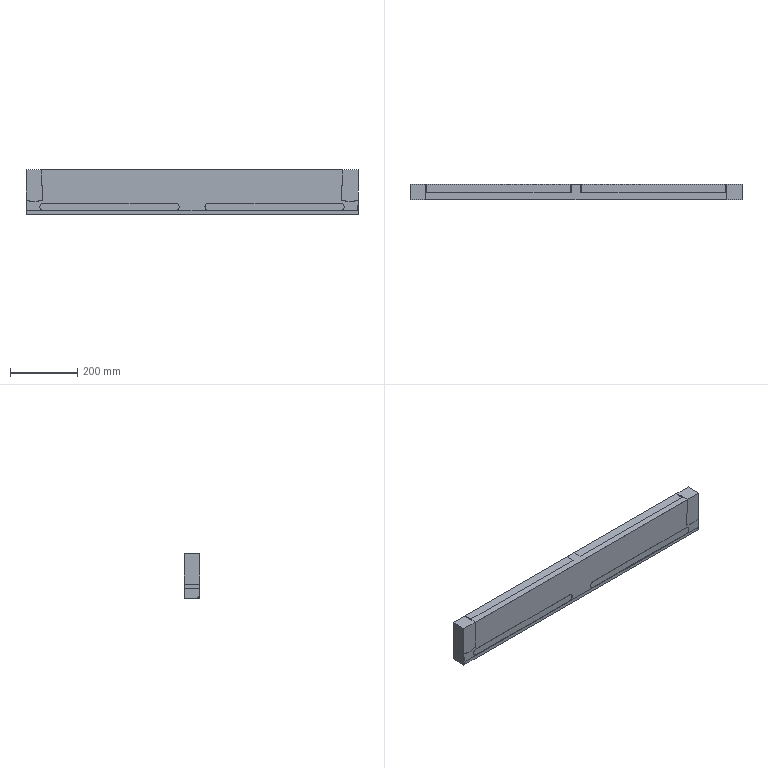NC program | NX | posted with a generic post | part box 987 x 45 x 132.5 mm
Whole program:
N10 G17 G21 G94 G90
(ZLEVEL_PROFILE_COPY_1 , TOOL : D12)
N12 T20 M6
N14 G54
N16 G17 G0 G90 X498.091 Y74.538 B0. C0. S7500 M3
N18 G43 Z30. H20
N20 Z-1.
N22 G94 G1 X496.514 Y73.404 F3000.
N24 G3 X496.021 Y72.311 R1.2
N26 G1 X496.534 Y67.184
N28 X496.619 Y66.359
N30 X499.57 Y36.857
N32 X499.6 Y36.25
N34 Y31.513
N36 X499.597 Y31.459
N38 Y20.192
N40 G3 X500.197 Y19.153 R1.2
N42 G1 X501.779 Y18.239
N44 G0 X501.78 Z-2.
N46 G1 X500.197 Y19.153
N48 G2 X499.597 Y20.192 R1.2
N50 G1 Y31.459
N52 X499.6 Y31.513
N54 Y36.25
N56 X499.57 Y36.857
N58 X496.619 Y66.359
N60 X496.534 Y67.184
N62 X496.021 Y72.311
N64 G2 X496.514 Y73.404 R1.2
N66 G1 X498.091 Y74.538
N68 G0 Z-3.
N70 G1 X496.514 Y73.404
N72 G3 X496.021 Y72.311 R1.2
N74 G1 X496.534 Y67.184
N76 X496.619 Y66.359
N78 X499.57 Y36.857
N80 X499.6 Y36.25
N82 Y31.513
N84 X499.597 Y31.459
N86 Y20.192
N88 G3 X500.197 Y19.153 R1.2
N90 G1 X501.78 Y18.239
N92 G0 Z-4.
N94 G1 X500.197 Y19.153
N96 G2 X499.597 Y20.192 R1.2
N98 G1 X499.6 Y31.513
N100 Y36.25
N102 X499.57 Y36.857
N104 X496.619 Y66.359
N106 X496.534 Y67.184
N108 X496.021 Y72.311
N110 G2 X496.514 Y73.404 R1.2
N112 G1 X498.092 Y74.538
N114 G0 Z-5.
N116 G1 X496.514 Y73.404
N118 G3 X496.021 Y72.311 R1.2
N120 G1 X496.534 Y67.184
N122 X496.619 Y66.359
N124 X499.57 Y36.857
N126 X499.6 Y36.25
N128 X499.597 Y31.459
N130 Y20.192
N132 G3 X500.197 Y19.153 R1.2
N134 G1 X501.78 Y18.239
N136 G0 Z-6.
N138 G1 X500.197 Y19.153
N140 G2 X499.597 Y20.192 R1.2
N142 G1 X499.6 Y31.513
N144 Y36.25
N146 X499.57 Y36.857
N148 X496.619 Y66.359
N150 X496.534 Y67.184
N152 X496.021 Y72.311
N154 G2 X496.515 Y73.404 R1.2
N156 G1 X498.092 Y74.538
N158 G0 Z-7.
N160 G1 X496.515 Y73.404
N162 G3 X496.021 Y72.311 R1.2
N164 G1 X496.534 Y67.184
N166 X496.619 Y66.359
N168 X499.57 Y36.857
N170 X499.6 Y36.25
N172 X499.597 Y31.459
N174 Y20.192
N176 G3 X500.197 Y19.153 R1.2
N178 G1 X501.78 Y18.239
N180 G0 Z-8.
N182 G1 X500.197 Y19.153
N184 G2 X499.597 Y20.192 R1.2
N186 G1 X499.6 Y31.513
N188 Y36.25
N190 X499.57 Y36.857
N192 X496.619 Y66.359
N194 X496.534 Y67.184
N196 X496.021 Y72.311
N198 G2 X496.515 Y73.404 R1.2
N200 G1 X498.092 Y74.538
N202 G0 Z-9.
N204 G1 X496.515 Y73.404
N206 G3 X496.021 Y72.311 R1.2
N208 G1 X496.534 Y67.184
N210 X496.619 Y66.359
N212 X499.57 Y36.857
N214 X499.6 Y36.25
N216 X499.597 Y31.459
N218 Y20.192
N220 G3 X500.197 Y19.153 R1.2
N222 G1 X501.78 Y18.239
N224 G0 Z-10.
N226 G1 X500.197 Y19.153
N228 G2 X499.597 Y20.192 R1.2
N230 G1 X499.6 Y31.513
N232 Y36.25
N234 X499.57 Y36.857
N236 X496.619 Y66.359
N238 X496.534 Y67.184
N240 X496.021 Y72.311
N242 G2 X496.515 Y73.404 R1.2
N244 G1 X498.092 Y74.538
N246 G0 Z-11.
N248 G1 X496.515 Y73.404
N250 G3 X496.021 Y72.311 R1.2
N252 G1 X496.534 Y67.184
N254 X496.619 Y66.359
N256 X499.57 Y36.857
N258 X499.6 Y36.25
N260 X499.597 Y31.459
N262 Y20.192
N264 G3 X500.197 Y19.153 R1.2
N266 G1 X501.78 Y18.239
N268 G0 Z-12.
N270 G1 X500.197 Y19.153
N272 G2 X499.597 Y20.192 R1.2
N274 G1 X499.6 Y31.513
N276 Y36.25
N278 X499.57 Y36.857
N280 X496.619 Y66.359
N282 X496.534 Y67.184
N284 X496.022 Y72.311
N286 G2 X496.515 Y73.405 R1.2
N288 G1 X498.092 Y74.538
N290 G0 Z-13.
N292 G1 X496.515 Y73.405
N294 G3 X496.022 Y72.311 R1.2
N296 G1 X496.535 Y67.184
N298 X496.619 Y66.359
N300 X499.57 Y36.857
N302 X499.6 Y36.25
N304 X499.598 Y31.459
N306 Y20.192
N308 G3 X500.198 Y19.153 R1.2
N310 G1 X501.78 Y18.239
N312 G0 Z-14.
N314 G1 X500.198 Y19.153
N316 G2 X499.598 Y20.192 R1.2
N318 G1 X499.6 Y31.513
N320 Y36.25
N322 X499.57 Y36.857
N324 X496.619 Y66.359
N326 X496.535 Y67.184
N328 X496.022 Y72.311
N330 G2 X496.515 Y73.405 R1.2
N332 G1 X498.092 Y74.538
N334 G0 X498.093 Z-15.
N336 G1 X496.515 Y73.405
N338 G3 X496.022 Y72.311 R1.2
N340 G1 X496.535 Y67.184
N342 X496.619 Y66.359
N344 X499.57 Y36.857
N346 X499.6 Y36.25
N348 X499.598 Y31.459
N350 Y20.192
N352 G3 X500.198 Y19.153 R1.2
N354 G1 X501.78 Y18.239
N356 G0 Z-16.
N358 G1 X500.198 Y19.153
N360 G2 X499.598 Y20.192 R1.2
N362 G1 X499.6 Y31.513
N364 Y36.25
N366 X499.57 Y36.857
N368 X496.619 Y66.359
N370 X496.535 Y67.184
N372 X496.022 Y72.311
N374 G2 X496.515 Y73.405 R1.2
N376 G1 X498.093 Y74.538
N378 G0 X498.092 Y74.539 Z-17.
N380 G1 X496.515 Y73.405
N382 G3 X496.022 Y72.311 R1.2
N384 G1 X496.619 Y66.359
N386 X499.57 Y36.857
N388 X499.6 Y36.25
N390 X499.598 Y31.459
N392 Y20.192
N394 G3 X500.198 Y19.153 R1.2
N396 G1 X501.78 Y18.239
N398 G0 Z-18.
N400 G1 X500.198 Y19.153
N402 G2 X499.598 Y20.192 R1.2
N404 G1 X499.6 Y31.513
N406 Y36.25
N408 X499.57 Y36.857
N410 X496.619 Y66.359
N412 X496.022 Y72.311
N414 G2 X496.515 Y73.405 R1.2
N416 G1 X498.092 Y74.539
N418 G0 X498.097 Y74.542 Z-19.
N420 G1 X496.515 Y73.405
N422 G3 X496.022 Y72.311 R1.2
N424 G1 X496.619 Y66.359
N426 X499.57 Y36.857
N428 X499.6 Y36.25
N430 X499.598 Y31.459
N432 Y20.192
N434 G3 X500.198 Y19.153 R1.2
N436 G1 X501.78 Y18.239
N438 G0 X501.781 Z-20.
N440 G1 X500.198 Y19.153
N442 G2 X499.598 Y20.192 R1.2
N444 G1 X499.6 Y31.513
N446 Y36.25
N448 X499.57 Y36.857
N450 X496.619 Y66.359
N452 X496.022 Y72.311
N454 G2 X496.515 Y73.405 R1.2
N456 G1 X498.097 Y74.542
N458 G0 Y74.541 Z-21.
N460 G1 X496.516 Y73.405
N462 G3 X496.022 Y72.311 R1.2
N464 G1 X496.535 Y67.184
N466 X496.619 Y66.359
N468 X499.57 Y36.857
N470 X499.6 Y36.25
N472 X499.598 Y31.459
N474 Y20.192
N476 G3 X500.198 Y19.153 R1.2
N478 G1 X501.781 Y18.239
N480 G0 Y18.238 Z-22.
N482 G1 X500.198 Y19.153
N484 G2 X499.598 Y20.192 R1.2
N486 G1 X499.6 Y31.513
N488 Y36.25
N490 X499.57 Y36.857
N492 X496.619 Y66.359
N494 X496.535 Y67.184
N496 X496.022 Y72.311
N498 G2 X496.516 Y73.405 R1.2
N500 G1 X498.097 Y74.541
N502 G0 Z-23.
N504 G1 X496.516 Y73.405
N506 G3 X496.023 Y72.311 R1.2
N508 G1 X496.535 Y67.184
N510 X496.619 Y66.359
N512 X499.57 Y36.857
N514 X499.6 Y36.25
N516 Y31.513
N518 X499.598 Y20.192
N520 G3 X500.198 Y19.153 R1.2
N522 G1 X501.781 Y18.238
N524 G0 Z-24.
N526 G1 X500.198 Y19.153
N528 G2 X499.598 Y20.192 R1.2
N530 G1 X499.6 Y31.513
N532 Y36.25
N534 X499.57 Y36.857
N536 X496.619 Y66.359
N538 X496.023 Y72.311
N540 G2 X496.516 Y73.405 R1.2
N542 G1 X498.097 Y74.542
N544 G0 Z-25.
N546 G1 X496.516 Y73.405
N548 G3 X496.023 Y72.311 R1.2
N550 G1 X496.619 Y66.359
N552 X499.57 Y36.857
N554 X499.6 Y36.25
N556 Y31.513
N558 X499.598 Y20.192
N560 G3 X500.198 Y19.153 R1.2
N562 G1 X501.781 Y18.239
N564 G0 Z-26.
N566 G1 X500.198 Y19.153
N568 G2 X499.598 Y20.192 R1.2
N570 G1 X499.6 Y31.513
N572 Y36.25
N574 X499.57 Y36.857
N576 X496.619 Y66.359
N578 X496.023 Y72.311
N580 G2 X496.516 Y73.405 R1.2
N582 G1 X498.097 Y74.542
N584 G0 Z-27.
N586 G1 X496.516 Y73.405
N588 G3 X496.023 Y72.311 R1.2
N590 G1 X496.619 Y66.359
N592 X499.57 Y36.857
N594 X499.6 Y36.25
N596 Y31.513
N598 X499.598 Y20.192
N600 G3 X500.198 Y19.153 R1.2
N602 G1 X501.781 Y18.239
N604 G0 Z-28.
N606 G1 X500.198 Y19.153
N608 G2 X499.599 Y20.192 R1.2
N610 G1 X499.6 Y31.513
N612 Y36.25
N614 X499.57 Y36.857
N616 X496.619 Y66.359
N618 X496.023 Y72.311
N620 G2 X496.516 Y73.405 R1.2
N622 G1 X498.097 Y74.542
N624 G0 Z-29.
N626 G1 X496.516 Y73.405
N628 G3 X496.023 Y72.311 R1.2
N630 G1 X496.619 Y66.359
N632 X499.57 Y36.857
N634 X499.6 Y36.25
N636 Y31.513
N638 X499.599 Y20.192
N640 G3 X500.198 Y19.153 R1.2
N642 G1 X501.781 Y18.239
N644 G0 Z-30.
N646 G1 X500.199 Y19.153
N648 G2 X499.599 Y20.192 R1.2
N650 G1 X499.6 Y31.513
N652 Y36.25
N654 X499.57 Y36.857
N656 X496.619 Y66.359
N658 X496.023 Y72.311
N660 G2 X496.517 Y73.405 R1.2
N662 G1 X498.097 Y74.542
N664 G0 Y74.541 Z-31.
N666 G1 X496.517 Y73.405
N668 G3 X496.023 Y72.311 R1.2
N670 G1 X496.619 Y66.359
N672 X499.57 Y36.857
N674 X499.6 Y36.25
N676 Y31.513
N678 X499.599 Y20.192
N680 G3 X500.199 Y19.153 R1.2
N682 G1 X501.781 Y18.239
N684 G0 Z-32.
N686 G1 X500.199 Y19.153
N688 G2 X499.599 Y20.192 R1.2
N690 G1 X499.6 Y31.513
N692 Y36.25
N694 X499.57 Y36.857
N696 X496.619 Y66.359
N698 X496.023 Y72.311
N700 G2 X496.517 Y73.405 R1.2
N702 G1 X498.097 Y74.541
N704 G0 Z-33.
N706 G1 X496.517 Y73.405
N708 G3 X496.023 Y72.311 R1.2
N710 G1 X496.619 Y66.359
N712 X499.57 Y36.857
N714 X499.6 Y36.25
N716 Y31.513
N718 X499.599 Y20.192
N720 G3 X500.199 Y19.153 R1.2
N722 G1 X501.781 Y18.239
N724 G0 Z-34.
N726 G1 X500.199 Y19.153
N728 G2 X499.599 Y20.192 R1.2
N730 G1 X499.6 Y31.513
N732 Y36.25
N734 X499.57 Y36.857
N736 X496.619 Y66.359
N738 X496.024 Y72.311
N740 G2 X496.517 Y73.405 R1.2
N742 G1 X498.097 Y74.541
N744 G0 Z-35.
N746 G1 X496.517 Y73.405
N748 G3 X496.024 Y72.311 R1.2
N750 G1 X496.619 Y66.359
N752 X499.57 Y36.857
N754 X499.6 Y36.25
N756 Y31.513
N758 X499.599 Y20.192
N760 G3 X500.199 Y19.153 R1.2
N762 G1 X501.781 Y18.239
N764 G0 Z-36.
N766 G1 X500.199 Y19.153
N768 G2 X499.599 Y20.192 R1.2
N770 G1 X499.6 Y31.513
N772 Y36.25
N774 X499.57 Y36.857
N776 X496.619 Y66.359
N778 X496.024 Y72.311
N780 G2 X496.517 Y73.405 R1.2
N782 G1 X498.098 Y74.541
N784 G0 X498.094 Y74.539 Z-37.
N786 G1 X496.517 Y73.405
N788 G3 X496.024 Y72.311 R1.2
N790 G1 X496.619 Y66.359
N792 X499.57 Y36.857
N794 X499.6 Y36.25
N796 Y31.513
N798 X499.599 Y20.192
N800 G3 X500.199 Y19.153 R1.2
N802 G1 X501.781 Y18.239
N804 G0 Z-38.
N806 G1 X500.199 Y19.153
N808 G2 X499.599 Y20.192 R1.2
N810 G1 X499.6 Y31.513
N812 Y36.25
N814 X499.57 Y36.857
N816 X496.619 Y66.359
N818 X496.024 Y72.311
N820 G2 X496.517 Y73.405 R1.2
N822 G1 X498.094 Y74.539
N824 G0 Y74.538 Z-39.
N826 G1 X496.518 Y73.405
N828 G3 X496.024 Y72.311 R1.2
N830 G1 X496.619 Y66.359
N832 X499.57 Y36.857
N834 X499.6 Y36.25
N836 Y31.513
N838 X499.599 Y20.192
N840 G3 X500.199 Y19.152 R1.2
N842 G1 X501.781 Y18.239
N844 G0 Z-40.
N846 G1 X500.199 Y19.152
N848 G2 X499.599 Y20.192 R1.2
N850 G1 X499.6 Y31.513
N852 Y36.25
N854 X499.57 Y36.857
N856 X496.619 Y66.359
N858 X496.024 Y72.311
N860 G2 X496.518 Y73.405 R1.2
N862 G1 X498.095 Y74.538
N864 G0 Z-41.
N866 G1 X496.518 Y73.405
N868 G3 X496.024 Y72.311 R1.2
N870 G1 X496.619 Y66.359
N872 X499.57 Y36.857
N874 X499.6 Y36.25
N876 Y31.513
N878 X499.599 Y20.192
N880 G3 X500.199 Y19.152 R1.2
N882 G1 X501.781 Y18.239
N884 G0 X501.782 Z-42.
N886 G1 X500.199 Y19.152
N888 G2 X499.599 Y20.192 R1.2
N890 G1 X499.6 Y31.513
N892 Y36.25
N894 X499.57 Y36.857
N896 X496.619 Y66.359
N898 X496.024 Y72.311
N900 G2 X496.518 Y73.405 R1.2
N902 G1 X498.095 Y74.538
N904 G0 Z-43.
N906 G1 X496.518 Y73.405
N908 G3 X496.024 Y72.311 R1.2
N910 G1 X496.619 Y66.359
N912 X499.57 Y36.857
N914 X499.6 Y36.25
N916 Y31.513
N918 X499.599 Y20.192
N920 G3 X500.199 Y19.152 R1.2
N922 G1 X501.782 Y18.239
N924 G0 Z-44.
N926 G1 X500.199 Y19.152
N928 G2 X499.6 Y20.192 R1.2
N930 G1 Y31.513
N932 Y36.25
N934 X499.57 Y36.857
N936 X496.619 Y66.359
N938 X496.024 Y72.311
N940 G2 X496.518 Y73.405 R1.2
N942 G1 X498.095 Y74.538
N944 G0 Z-45.
N946 G1 X496.518 Y73.405
N948 G3 X496.024 Y72.311 R1.2
N950 G1 X496.619 Y66.359
N952 X499.57 Y36.857
N954 X499.6 Y36.25
N956 Y31.513
N958 Y20.192
N960 G3 X500.2 Y19.152 R1.2
N962 G1 X501.782 Y18.239
N964 G0 Z30.
N966 X-501.779
N968 Z-1.
N970 G1 X-500.197 Y19.153
N972 G3 X-499.597 Y20.192 R1.2
N974 G1 Y25.852
N976 X-499.542 Y25.913
N978 G2 X-499.54 Y27.606 R6.1
N980 G1 X-499.597 Y27.668
N982 Y31.459
N984 X-499.6 Y31.513
N986 Y36.25
N988 X-499.57 Y36.857
N990 X-496.619 Y66.359
N992 X-496.477 Y67.194
N994 X-496.528 Y67.237
N996 X-496.021 Y72.311
N998 G3 X-496.514 Y73.404 R1.2
N1000 G1 X-498.098 Y74.543
N1002 G0 Z-2.
N1004 G1 X-496.514 Y73.404
N1006 G2 X-496.021 Y72.311 R1.2
N1008 G1 X-496.528 Y67.237
N1010 X-496.477 Y67.194
N1012 X-496.619 Y66.359
N1014 X-499.57 Y36.857
N1016 X-499.6 Y36.25
N1018 Y31.513
N1020 X-499.597 Y31.459
N1022 Y27.668
N1024 X-499.54 Y27.606
N1026 G3 X-499.542 Y25.913 R6.1
N1028 G1 X-499.597 Y25.852
N1030 Y20.192
N1032 G2 X-500.197 Y19.153 R1.2
N1034 G1 X-501.78 Y18.239
N1036 G0 Z-3.
N1038 G1 X-500.197 Y19.153
N1040 G3 X-499.597 Y20.192 R1.2
N1042 G1 Y25.852
N1044 X-499.542 Y25.913
N1046 G2 X-499.54 Y27.606 R6.1
N1048 G1 X-499.597 Y27.668
N1050 Y31.459
N1052 X-499.6 Y31.513
N1054 Y36.25
N1056 X-499.57 Y36.857
N1058 X-496.619 Y66.359
N1060 X-496.477 Y67.194
N1062 X-496.529 Y67.237
N1064 X-496.021 Y72.311
N1066 G3 X-496.514 Y73.404 R1.2
N1068 G1 X-498.098 Y74.543
N1070 G0 Z-4.
N1072 G1 X-496.514 Y73.404
N1074 G2 X-496.021 Y72.311 R1.2
N1076 G1 X-496.529 Y67.237
N1078 X-496.477 Y67.194
N1080 X-496.619 Y66.359
N1082 X-499.57 Y36.857
N1084 X-499.6 Y36.25
N1086 X-499.597 Y31.459
N1088 Y27.668
N1090 X-499.54 Y27.606
N1092 G3 X-499.542 Y25.913 R6.1
N1094 G1 X-499.597 Y25.852
N1096 Y20.192
N1098 G2 X-500.197 Y19.153 R1.2
N1100 G1 X-501.78 Y18.239
N1102 G0 Z-5.
N1104 G1 X-500.197 Y19.153
N1106 G3 X-499.597 Y20.192 R1.2
N1108 G1 Y25.852
N1110 X-499.542 Y25.913
N1112 G2 X-499.54 Y27.606 R6.1
N1114 G1 X-499.597 Y27.668
N1116 X-499.6 Y31.513
N1118 Y36.25
N1120 X-499.57 Y36.857
N1122 X-496.619 Y66.359
N1124 X-496.477 Y67.194
N1126 X-496.529 Y67.237
N1128 X-496.021 Y72.311
N1130 G3 X-496.514 Y73.404 R1.2
N1132 G1 X-498.098 Y74.543
N1134 G0 Z-6.
N1136 G1 X-496.515 Y73.404
N1138 G2 X-496.021 Y72.311 R1.2
N1140 G1 X-496.529 Y67.237
N1142 X-496.477 Y67.194
N1144 X-496.619 Y66.359
N1146 X-499.57 Y36.857
N1148 X-499.6 Y36.25
N1150 X-499.597 Y31.459
N1152 Y27.668
N1154 X-499.54 Y27.606
N1156 G3 X-499.542 Y25.913 R6.1
N1158 G1 X-499.597 Y25.852
N1160 Y20.192
N1162 G2 X-500.197 Y19.153 R1.2
N1164 G1 X-501.78 Y18.239
N1166 G0 Z-7.
N1168 G1 X-500.197 Y19.153
N1170 G3 X-499.597 Y20.192 R1.2
N1172 G1 Y25.852
N1174 X-499.542 Y25.913
N1176 G2 X-499.54 Y27.606 R6.1
N1178 G1 X-499.597 Y27.668
N1180 X-499.6 Y31.513
N1182 Y36.25
N1184 X-499.57 Y36.857
N1186 X-496.619 Y66.359
N1188 X-496.477 Y67.194
N1190 X-496.529 Y67.237
N1192 X-496.021 Y72.311
N1194 G3 X-496.515 Y73.404 R1.2
N1196 G1 X-498.098 Y74.543
N1198 G0 Z-8.
N1200 G1 X-496.515 Y73.404
N1202 G2 X-496.021 Y72.311 R1.2
N1204 G1 X-496.529 Y67.237
N1206 X-496.477 Y67.194
N1208 X-496.619 Y66.359
N1210 X-499.57 Y36.857
N1212 X-499.6 Y36.25
N1214 X-499.597 Y31.459
N1216 Y27.668
N1218 X-499.54 Y27.606
N1220 G3 X-499.542 Y25.913 R6.1
N1222 G1 X-499.597 Y25.852
N1224 Y20.192
N1226 G2 X-500.197 Y19.153 R1.2
N1228 G1 X-501.78 Y18.239
N1230 G0 Z-9.
N1232 G1 X-500.197 Y19.153
N1234 G3 X-499.597 Y20.192 R1.2
N1236 G1 Y25.852
N1238 X-499.542 Y25.913
N1240 G2 X-499.54 Y27.606 R6.1
N1242 G1 X-499.597 Y27.668
N1244 X-499.6 Y31.513
N1246 Y36.25
N1248 X-499.57 Y36.857
N1250 X-496.619 Y66.359
N1252 X-496.477 Y67.194
N1254 X-496.529 Y67.237
N1256 X-496.021 Y72.311
N1258 G3 X-496.515 Y73.404 R1.2
N1260 G1 X-498.099 Y74.543
N1262 G0 Z-10.
N1264 G1 X-496.515 Y73.404
N1266 G2 X-496.021 Y72.311 R1.2
N1268 G1 X-496.529 Y67.237
N1270 X-496.477 Y67.194
N1272 X-496.619 Y66.359
N1274 X-499.57 Y36.857
N1276 X-499.6 Y36.25
N1278 X-499.597 Y31.459
N1280 Y27.668
N1282 X-499.54 Y27.606
N1284 G3 X-499.542 Y25.913 R6.1
N1286 G1 X-499.597 Y25.852
N1288 Y20.192
N1290 G2 X-500.197 Y19.153 R1.2
N1292 G1 X-501.78 Y18.239
N1294 G0 Z-11.
N1296 G1 X-500.197 Y19.153
N1298 G3 X-499.597 Y20.192 R1.2
N1300 G1 Y25.852
N1302 X-499.542 Y25.913
N1304 G2 X-499.54 Y27.606 R6.1
N1306 G1 X-499.597 Y27.668
N1308 X-499.6 Y31.513
N1310 Y36.25
N1312 X-499.57 Y36.857
N1314 X-496.619 Y66.359
N1316 X-496.477 Y67.194
N1318 X-496.529 Y67.237
N1320 X-496.021 Y72.311
N1322 G3 X-496.515 Y73.404 R1.2
N1324 G1 X-498.099 Y74.543
N1326 G0 Z-12.
N1328 G1 X-496.515 Y73.405
N1330 G2 X-496.022 Y72.311 R1.2
N1332 G1 X-496.529 Y67.237
N1334 X-496.477 Y67.194
N1336 X-496.619 Y66.359
N1338 X-499.57 Y36.857
N1340 X-499.6 Y36.25
N1342 X-499.598 Y31.459
N1344 Y27.668
N1346 X-499.54 Y27.606
N1348 G3 X-499.542 Y25.913 R6.1
N1350 G1 X-499.598 Y25.852
N1352 X-499.597 Y20.192
N1354 G2 X-500.197 Y19.153 R1.2
N1356 G1 X-501.78 Y18.239
N1358 G0 Z-13.
N1360 G1 X-500.198 Y19.153
N1362 G3 X-499.598 Y20.192 R1.2
N1364 G1 Y25.852
N1366 X-499.542 Y25.913
N1368 G2 X-499.54 Y27.606 R6.1
N1370 G1 X-499.598 Y27.668
N1372 X-499.6 Y31.513
N1374 Y36.25
N1376 X-499.57 Y36.857
N1378 X-496.619 Y66.359
N1380 X-496.477 Y67.194
N1382 X-496.529 Y67.237
N1384 X-496.022 Y72.311
N1386 G3 X-496.515 Y73.405 R1.2
N1388 G1 X-498.099 Y74.543
N1390 G0 Z-14.
N1392 G1 X-496.515 Y73.405
N1394 G2 X-496.022 Y72.311 R1.2
N1396 G1 X-496.529 Y67.237
N1398 X-496.477 Y67.194
N1400 X-496.619 Y66.359
N1402 X-499.57 Y36.857
N1404 X-499.6 Y36.25
N1406 X-499.598 Y31.459
N1408 Y27.668
N1410 X-499.54 Y27.606
N1412 G3 X-499.542 Y25.913 R6.1
N1414 G1 X-499.598 Y25.852
N1416 Y20.192
N1418 G2 X-500.198 Y19.153 R1.2
N1420 G1 X-501.78 Y18.239
N1422 G0 Z-15.
N1424 G1 X-500.198 Y19.153
N1426 G3 X-499.598 Y20.192 R1.2
N1428 G1 Y25.852
N1430 X-499.542 Y25.913
N1432 G2 X-499.54 Y27.606 R6.1
N1434 G1 X-499.598 Y27.668
N1436 X-499.6 Y31.513
N1438 Y36.25
N1440 X-499.57 Y36.857
N1442 X-496.619 Y66.359
N1444 X-496.477 Y67.194
N1446 X-496.529 Y67.237
N1448 X-496.022 Y72.311
N1450 G3 X-496.515 Y73.405 R1.2
N1452 G1 X-498.099 Y74.543
N1454 G0 Z-16.
N1456 G1 X-496.515 Y73.405
N1458 G2 X-496.022 Y72.311 R1.2
N1460 G1 X-496.529 Y67.237
N1462 X-496.477 Y67.194
N1464 X-496.619 Y66.359
N1466 X-499.57 Y36.857
N1468 X-499.6 Y36.25
N1470 X-499.598 Y31.459
N1472 Y27.668
N1474 X-499.54 Y27.606
N1476 G3 X-499.542 Y25.913 R6.1
N1478 G1 X-499.598 Y25.852
N1480 Y20.192
N1482 G2 X-500.198 Y19.153 R1.2
N1484 G1 X-501.78 Y18.239
N1486 G0 Z-17.
N1488 G1 X-500.198 Y19.153
N1490 G3 X-499.598 Y20.192 R1.2
N1492 G1 Y25.852
N1494 X-499.542 Y25.913
N1496 G2 X-499.54 Y27.606 R6.1
N1498 G1 X-499.598 Y27.668
N1500 X-499.6 Y31.513
N1502 Y36.25
N1504 X-499.57 Y36.857
N1506 X-496.619 Y66.359
N1508 X-496.477 Y67.194
N1510 X-496.53 Y67.237
N1512 X-496.022 Y72.311
N1514 G3 X-496.516 Y73.405 R1.2
N1516 G1 X-498.099 Y74.543
N1518 G0 Z-18.
N1520 G1 X-496.516 Y73.405
N1522 G2 X-496.022 Y72.311 R1.2
N1524 G1 X-496.53 Y67.237
N1526 X-496.477 Y67.194
N1528 X-496.619 Y66.359
N1530 X-499.57 Y36.857
N1532 X-499.6 Y36.25
N1534 X-499.598 Y31.459
N1536 Y27.668
N1538 X-499.54 Y27.606
N1540 G3 X-499.542 Y25.913 R6.1
N1542 G1 X-499.598 Y25.852
N1544 Y20.192
N1546 G2 X-500.198 Y19.153 R1.2
N1548 G1 X-501.78 Y18.239
N1550 G0 Z-19.
N1552 G1 X-500.198 Y19.153
N1554 G3 X-499.598 Y20.192 R1.2
N1556 G1 Y25.852
N1558 X-499.542 Y25.913
N1560 G2 X-499.54 Y27.606 R6.1
N1562 G1 X-499.598 Y27.668
N1564 X-499.6 Y31.513
N1566 Y36.25
N1568 X-499.57 Y36.857
N1570 X-496.619 Y66.359
N1572 X-496.477 Y67.194
N1574 X-496.53 Y67.237
N1576 X-496.022 Y72.311
N1578 G3 X-496.516 Y73.405 R1.2
N1580 G1 X-498.099 Y74.543
N1582 G0 Z-20.
N1584 G1 X-496.516 Y73.405
N1586 G2 X-496.022 Y72.311 R1.2
N1588 G1 X-496.53 Y67.237
N1590 X-496.477 Y67.194
N1592 X-496.619 Y66.359
N1594 X-499.57 Y36.857
N1596 X-499.6 Y36.25
N1598 X-499.598 Y31.459
N1600 Y27.668
N1602 X-499.54 Y27.606
N1604 G3 X-499.542 Y25.913 R6.1
N1606 G1 X-499.598 Y25.852
N1608 Y20.192
N1610 G2 X-500.198 Y19.153 R1.2
N1612 G1 X-501.781 Y18.239
N1614 G0 Z-21.
N1616 G1 X-500.198 Y19.153
N1618 G3 X-499.598 Y20.192 R1.2
N1620 G1 Y25.852
N1622 X-499.542 Y25.913
N1624 G2 X-499.54 Y27.606 R6.1
N1626 G1 X-499.598 Y27.668
N1628 X-499.6 Y31.513
N1630 Y36.25
N1632 X-499.57 Y36.857
N1634 X-496.619 Y66.359
N1636 X-496.477 Y67.194
N1638 X-496.53 Y67.237
N1640 X-496.022 Y72.311
N1642 G3 X-496.516 Y73.405 R1.2
N1644 G1 X-498.099 Y74.543
N1646 G0 X-498.1 Z-22.
N1648 G1 X-496.516 Y73.405
N1650 G2 X-496.022 Y72.311 R1.2
N1652 G1 X-496.53 Y67.237
N1654 X-496.477 Y67.194
N1656 X-496.619 Y66.359
N1658 X-499.57 Y36.857
N1660 X-499.6 Y36.25
N1662 Y31.513
N1664 X-499.598 Y27.668
N1666 X-499.54 Y27.606
N1668 G3 X-499.542 Y25.913 R6.1
N1670 G1 X-499.598 Y25.852
N1672 Y20.192
N1674 G2 X-500.198 Y19.153 R1.2
N1676 G1 X-501.781 Y18.239
N1678 G0 Z-23.
N1680 G1 X-500.198 Y19.153
N1682 G3 X-499.598 Y20.192 R1.2
N1684 G1 Y25.852
N1686 X-499.542 Y25.913
N1688 G2 X-499.54 Y27.606 R6.1
N1690 G1 X-499.598 Y27.668
N1692 X-499.6 Y31.513
N1694 Y36.25
N1696 X-499.57 Y36.857
N1698 X-496.619 Y66.359
N1700 X-496.477 Y67.194
N1702 X-496.53 Y67.237
N1704 X-496.023 Y72.311
N1706 G3 X-496.516 Y73.405 R1.2
N1708 G1 X-498.1 Y74.543
N1710 G0 Z-24.
N1712 G1 X-496.516 Y73.405
N1714 G2 X-496.023 Y72.311 R1.2
N1716 G1 X-496.53 Y67.237
N1718 X-496.477 Y67.194
N1720 X-496.619 Y66.359
N1722 X-499.57 Y36.857
N1724 X-499.6 Y36.25
N1726 Y31.513
N1728 X-499.598 Y27.668
N1730 X-499.54 Y27.606
N1732 G3 X-499.542 Y25.913 R6.1
N1734 G1 X-499.598 Y25.852
N1736 Y20.192
N1738 G2 X-500.198 Y19.153 R1.2
N1740 G1 X-501.781 Y18.239
N1742 G0 Z-25.
N1744 G1 X-500.198 Y19.153
N1746 G3 X-499.598 Y20.192 R1.2
N1748 G1 Y25.852
N1750 X-499.542 Y25.913
N1752 G2 X-499.54 Y27.606 R6.1
N1754 G1 X-499.598 Y27.668
N1756 X-499.6 Y31.513
N1758 Y36.25
N1760 X-499.57 Y36.857
N1762 X-496.619 Y66.359
N1764 X-496.477 Y67.194
N1766 X-496.53 Y67.237
N1768 X-496.023 Y72.311
N1770 G3 X-496.516 Y73.405 R1.2
N1772 G1 X-498.1 Y74.543
N1774 G0 Z-26.
N1776 G1 X-496.516 Y73.405
N1778 G2 X-496.023 Y72.311 R1.2
N1780 G1 X-496.53 Y67.237
N1782 X-496.477 Y67.194
N1784 X-496.619 Y66.359
N1786 X-499.57 Y36.857
N1788 X-499.6 Y36.25
N1790 Y31.513
N1792 X-499.598 Y27.668
N1794 X-499.54 Y27.606
N1796 G3 X-499.542 Y25.913 R6.1
N1798 G1 X-499.598 Y25.852
N1800 Y20.192
N1802 G2 X-500.198 Y19.153 R1.2
N1804 G1 X-501.781 Y18.239
N1806 G0 Z-27.
N1808 G1 X-500.198 Y19.153
N1810 G3 X-499.598 Y20.192 R1.2
N1812 G1 Y25.852
N1814 X-499.542 Y25.913
N1816 G2 X-499.54 Y27.606 R6.1
N1818 G1 X-499.598 Y27.668
N1820 X-499.6 Y31.513
N1822 Y36.25
N1824 X-499.57 Y36.857
N1826 X-496.619 Y66.359
N1828 X-496.477 Y67.194
N1830 X-496.53 Y67.237
N1832 X-496.023 Y72.311
N1834 G3 X-496.517 Y73.405 R1.2
N1836 G1 X-498.1 Y74.543
N1838 G0 Z-28.
N1840 G1 X-496.517 Y73.405
N1842 G2 X-496.023 Y72.311 R1.2
N1844 G1 X-496.53 Y67.237
N1846 X-496.477 Y67.194
N1848 X-496.619 Y66.359
N1850 X-499.57 Y36.857
N1852 X-499.6 Y36.25
N1854 Y31.513
N1856 X-499.599 Y27.668
N1858 X-499.54 Y27.606
N1860 G3 X-499.542 Y25.913 R6.1
N1862 G1 X-499.599 Y25.852
N1864 Y20.192
N1866 G2 X-500.199 Y19.153 R1.2
N1868 G1 X-501.781 Y18.239
N1870 G0 Z-29.
N1872 G1 X-500.199 Y19.153
N1874 G3 X-499.599 Y20.192 R1.2
N1876 G1 Y25.852
N1878 X-499.542 Y25.913
N1880 G2 X-499.54 Y27.606 R6.1
N1882 G1 X-499.599 Y27.668
N1884 X-499.6 Y31.513
N1886 Y36.25
N1888 X-499.57 Y36.857
N1890 X-496.619 Y66.359
N1892 X-496.477 Y67.194
N1894 X-496.53 Y67.237
N1896 X-496.023 Y72.311
N1898 G3 X-496.517 Y73.405 R1.2
N1900 G1 X-498.1 Y74.543
N1902 G0 Z-30.
N1904 G1 X-496.517 Y73.405
N1906 G2 X-496.023 Y72.311 R1.2
N1908 G1 X-496.53 Y67.237
N1910 X-496.477 Y67.194
N1912 X-496.619 Y66.359
N1914 X-499.57 Y36.857
N1916 X-499.6 Y36.25
N1918 Y31.513
N1920 X-499.599 Y27.668
N1922 X-499.54 Y27.606
N1924 G3 X-499.542 Y25.913 R6.1
N1926 G1 X-499.599 Y25.852
N1928 Y20.192
N1930 G2 X-500.199 Y19.153 R1.2
N1932 G1 X-501.781 Y18.239
N1934 G0 Z-31.
N1936 G1 X-500.199 Y19.153
N1938 G3 X-499.599 Y20.192 R1.2
N1940 G1 Y25.852
N1942 X-499.542 Y25.913
N1944 G2 X-499.54 Y27.606 R6.1
N1946 G1 X-499.599 Y27.668
N1948 X-499.6 Y31.513
N1950 Y36.25
N1952 X-499.57 Y36.857
N1954 X-496.619 Y66.359
N1956 X-496.477 Y67.194
N1958 X-496.53 Y67.237
N1960 X-496.023 Y72.311
N1962 G3 X-496.517 Y73.405 R1.2
N1964 G1 X-498.1 Y74.543
N1966 G0 Z-32.
N1968 G1 X-496.517 Y73.405
N1970 G2 X-496.023 Y72.311 R1.2
N1972 G1 X-496.531 Y67.237
N1974 X-496.477 Y67.194
N1976 X-496.619 Y66.359
N1978 X-499.57 Y36.857
N1980 X-499.6 Y36.25
N1982 Y31.513
N1984 X-499.599 Y27.668
N1986 X-499.54 Y27.606
N1988 G3 X-499.542 Y25.913 R6.1
N1990 G1 X-499.599 Y25.852
N1992 Y20.192
N1994 G2 X-500.199 Y19.153 R1.2
N1996 G1 X-501.781 Y18.239
N1998 G0 Z-33.
N2000 G1 X-500.199 Y19.153
N2002 G3 X-499.599 Y20.192 R1.2
N2004 G1 Y25.852
N2006 X-499.542 Y25.913
N2008 G2 X-499.54 Y27.606 R6.1
N2010 G1 X-499.599 Y27.668
N2012 X-499.6 Y31.513
N2014 Y36.25
N2016 X-499.57 Y36.857
N2018 X-496.619 Y66.359
N2020 X-496.477 Y67.194
N2022 X-496.531 Y67.237
N2024 X-496.023 Y72.311
N2026 G3 X-496.517 Y73.405 R1.2
N2028 G1 X-498.1 Y74.543
N2030 G0 Z-34.
N2032 G1 X-496.517 Y73.405
N2034 G2 X-496.024 Y72.311 R1.2
N2036 G1 X-496.531 Y67.237
N2038 X-496.477 Y67.194
N2040 X-496.619 Y66.359
N2042 X-499.57 Y36.857
N2044 X-499.6 Y36.25
N2046 Y31.513
N2048 X-499.599 Y27.668
N2050 X-499.54 Y27.606
N2052 G3 X-499.542 Y25.913 R6.1
N2054 G1 X-499.599 Y25.852
N2056 Y20.192
N2058 G2 X-500.199 Y19.153 R1.2
N2060 G1 X-501.781 Y18.239
N2062 G0 Z-35.
N2064 G1 X-500.199 Y19.153
N2066 G3 X-499.599 Y20.192 R1.2
N2068 G1 Y25.852
N2070 X-499.542 Y25.913
N2072 G2 X-499.54 Y27.606 R6.1
N2074 G1 X-499.599 Y27.668
N2076 X-499.6 Y31.513
N2078 Y36.25
N2080 X-499.57 Y36.857
N2082 X-496.619 Y66.359
N2084 X-496.477 Y67.194
N2086 X-496.531 Y67.237
N2088 X-496.024 Y72.311
N2090 G3 X-496.517 Y73.405 R1.2
N2092 G1 X-498.101 Y74.543
N2094 G0 Z-36.
N2096 G1 X-496.517 Y73.405
N2098 G2 X-496.024 Y72.311 R1.2
N2100 G1 X-496.531 Y67.237
N2102 X-496.477 Y67.194
N2104 X-496.619 Y66.359
N2106 X-499.57 Y36.857
N2108 X-499.6 Y36.25
N2110 Y31.513
N2112 X-499.599 Y27.668
N2114 X-499.54 Y27.606
N2116 G3 X-499.542 Y25.913 R6.1
N2118 G1 X-499.599 Y25.852
N2120 Y20.192
N2122 G2 X-500.199 Y19.153 R1.2
N2124 G1 X-501.781 Y18.239
N2126 G0 Z-37.
N2128 G1 X-500.199 Y19.153
N2130 G3 X-499.599 Y20.192 R1.2
N2132 G1 Y25.852
N2134 X-499.542 Y25.913
N2136 G2 X-499.54 Y27.606 R6.1
N2138 G1 X-499.599 Y27.668
N2140 X-499.6 Y31.513
N2142 Y36.25
N2144 X-499.57 Y36.857
N2146 X-496.619 Y66.359
N2148 X-496.477 Y67.194
N2150 X-496.531 Y67.237
N2152 X-496.024 Y72.311
N2154 G3 X-496.517 Y73.405 R1.2
N2156 G1 X-498.101 Y74.543
N2158 G0 Z-38.
N2160 G1 X-496.518 Y73.405
N2162 G2 X-496.024 Y72.311 R1.2
N2164 G1 X-496.531 Y67.237
N2166 X-496.477 Y67.194
N2168 X-496.619 Y66.359
N2170 X-499.57 Y36.857
N2172 X-499.6 Y36.25
N2174 Y31.513
N2176 X-499.599 Y27.668
N2178 X-499.54 Y27.606
N2180 G3 X-499.542 Y25.913 R6.1
N2182 G1 X-499.599 Y25.852
N2184 Y20.192
N2186 G2 X-500.199 Y19.153 R1.2
N2188 G1 X-501.781 Y18.239
N2190 G0 Z-39.
N2192 G1 X-500.199 Y19.153
N2194 G3 X-499.599 Y20.192 R1.2
N2196 G1 Y25.852
N2198 X-499.542 Y25.913
N2200 G2 X-499.54 Y27.606 R6.1
N2202 G1 X-499.599 Y27.668
N2204 X-499.6 Y31.513
N2206 Y36.25
N2208 X-499.57 Y36.857
N2210 X-496.619 Y66.359
N2212 X-496.477 Y67.194
N2214 X-496.531 Y67.237
N2216 X-496.024 Y72.311
N2218 G3 X-496.518 Y73.405 R1.2
N2220 G1 X-498.101 Y74.543
N2222 G0 Z-40.
N2224 G1 X-496.518 Y73.405
N2226 G2 X-496.024 Y72.311 R1.2
N2228 G1 X-496.531 Y67.237
N2230 X-496.477 Y67.194
N2232 X-496.619 Y66.359
N2234 X-499.57 Y36.857
N2236 X-499.6 Y36.25
N2238 Y31.513
N2240 X-499.599 Y27.668
N2242 X-499.54 Y27.606
N2244 G3 X-499.542 Y25.913 R6.1
N2246 G1 X-499.599 Y25.852
N2248 Y20.192
N2250 G2 X-500.199 Y19.153 R1.2
N2252 G1 X-501.781 Y18.239
N2254 G0 Z-41.
N2256 G1 X-500.199 Y19.153
N2258 G3 X-499.599 Y20.192 R1.2
N2260 G1 Y25.852
N2262 X-499.542 Y25.913
N2264 G2 X-499.54 Y27.606 R6.1
N2266 G1 X-499.599 Y27.668
N2268 X-499.6 Y31.513
N2270 Y36.25
N2272 X-499.57 Y36.857
N2274 X-496.619 Y66.359
N2276 X-496.477 Y67.194
N2278 X-496.531 Y67.237
N2280 X-496.024 Y72.311
N2282 G3 X-496.518 Y73.405 R1.2
N2284 G1 X-498.101 Y74.543
N2286 G0 Z-42.
N2288 G1 X-496.518 Y73.405
N2290 G2 X-496.024 Y72.311 R1.2
N2292 G1 X-496.531 Y67.237
N2294 X-496.477 Y67.194
N2296 X-496.619 Y66.359
N2298 X-499.57 Y36.857
N2300 X-499.6 Y36.25
N2302 Y31.513
N2304 X-499.599 Y27.668
N2306 X-499.54 Y27.606
N2308 G3 X-499.542 Y25.913 R6.1
N2310 G1 X-499.599 Y25.852
N2312 Y20.192
N2314 G2 X-500.199 Y19.153 R1.2
N2316 G1 X-501.782 Y18.239
N2318 G0 Z-43.
N2320 G1 X-500.199 Y19.153
N2322 G3 X-499.599 Y20.192 R1.2
N2324 G1 Y25.852
N2326 X-499.542 Y25.913
N2328 G2 X-499.54 Y27.606 R6.1
N2330 G1 X-499.599 Y27.668
N2332 X-499.6 Y31.513
N2334 Y36.25
N2336 X-499.57 Y36.857
N2338 X-496.619 Y66.359
N2340 X-496.477 Y67.194
N2342 X-496.531 Y67.237
N2344 X-496.024 Y72.311
N2346 G3 X-496.518 Y73.405 R1.2
N2348 G1 X-498.101 Y74.543
N2350 G0 Z-44.
N2352 G1 X-496.518 Y73.405
N2354 G2 X-496.024 Y72.311 R1.2
N2356 G1 X-496.531 Y67.237
N2358 X-496.477 Y67.194
N2360 X-496.619 Y66.359
N2362 X-499.57 Y36.857
N2364 X-499.6 Y36.25
N2366 Y31.513
N2368 Y27.668
N2370 X-499.54 Y27.606
N2372 G3 X-499.542 Y25.913 R6.1
N2374 G1 X-499.6 Y25.852
N2376 Y20.192
N2378 G2 X-500.2 Y19.153 R1.2
N2380 G1 X-501.782 Y18.239
N2382 G0 Z-45.
N2384 G1 X-500.2 Y19.153
N2386 G3 X-499.6 Y20.192 R1.2
N2388 G1 Y25.852
N2390 X-499.542 Y25.913
N2392 G2 X-499.54 Y27.606 R6.1
N2394 G1 X-499.6 Y27.668
N2396 Y31.513
N2398 Y36.25
N2400 X-499.57 Y36.857
N2402 X-496.619 Y66.359
N2404 X-496.477 Y67.194
N2406 X-496.531 Y67.237
N2408 X-496.024 Y72.311
N2410 G3 X-496.518 Y73.405 R1.2
N2412 G1 X-498.101 Y74.543
N2414 G0 Z30.
N2416 M5
(111 , TOOL : D12JING)
N2418 T21 M6
N2420 G54
N2422 G17 G0 G90 X489.819 Y77.751 B0. C0. S6500 M3
N2424 G43 Z30. H21
N2426 Z-14.
N2428 G94 G1 Z-15. F1000.
N2430 G41 X489.752 Y77.677 D21
N2432 X489.041 Y76.545
N2434 G3 X489.252 Y75.017 R1.2
N2436 G1 X494.026 Y70.699
N2438 X494.576 Y70.201
N2440 G2 X496.52 Y66.35 R6.
N2442 G1 X499.47 Y36.847
N2444 G2 X499.5 Y36.25 R6.
N2446 G1 Y26.75
N2448 G2 X497.743 Y22.507 R6.
N2450 G1 X497.243 Y22.007
N2452 X492.716 Y17.483
N2454 G3 X492.581 Y15.947 R1.2
N2456 G1 X493.351 Y14.846
N2458 G40
N2460 X493.421 Y14.775
N2462 Z-14.
N2464 G0 Z30.
N2466 X489.82 Y77.752
N2468 Z-29.
N2470 G1 Z-30.
N2472 G41 X489.753 Y77.678
N2474 X489.042 Y76.545
N2476 G3 X489.253 Y75.017 R1.2
N2478 G1 X494.026 Y70.699
N2480 X494.576 Y70.201
N2482 G2 X496.52 Y66.35 R6.
N2484 G1 X499.47 Y36.847
N2486 G2 X499.5 Y36.25 R6.
N2488 G1 Y26.75
N2490 G2 X497.743 Y22.507 R6.
N2492 G1 X497.243 Y22.007
N2494 X492.716 Y17.483
N2496 G3 X492.581 Y15.946 R1.2
N2498 G1 X493.351 Y14.846
N2500 G40
N2502 X493.422 Y14.775
N2504 Z-29.
N2506 G0 Z30.
N2508 X489.821 Y77.752
N2510 Z-44.
N2512 G1 Z-45.
N2514 G41 X489.754 Y77.678
N2516 X489.042 Y76.545
N2518 G3 X489.253 Y75.017 R1.2
N2520 G1 X494.026 Y70.699
N2522 X494.576 Y70.201
N2524 G2 X496.52 Y66.35 R6.
N2526 G1 X499.47 Y36.847
N2528 G2 X499.5 Y36.25 R6.
N2530 G1 Y26.75
N2532 G2 X497.743 Y22.507 R6.
N2534 G1 X497.243 Y22.007
N2536 X496.977 Y21.744
N2538 X492.716 Y17.483
N2540 G3 X492.582 Y15.946 R1.2
N2542 G1 X493.352 Y14.846
N2544 G40
N2546 X493.423 Y14.775
N2548 Z-44.
N2550 G0 Z30.
N2552 X-493.423 Y14.776
N2554 Z-14.
N2556 G1 Z-15.
N2558 G41 X-493.352 Y14.846
N2560 X-492.582 Y15.946
N2562 G3 X-492.716 Y17.483 R1.2
N2564 G1 X-497.486 Y22.254
N2566 X-497.495 Y22.26
N2568 X-497.743 Y22.507
N2570 G2 X-499.489 Y27.113 R6.
N2572 G1 X-499.498 Y27.128
N2574 Y27.372
N2576 X-499.5 Y27.387
N2578 Y36.25
N2580 X-499.47 Y36.847
N2582 X-496.52 Y66.35
N2584 G2 X-494.576 Y70.201 R6.
N2586 G1 X-494.016 Y70.707
N2588 X-489.253 Y75.017
N2590 G3 X-489.042 Y76.545 R1.2
N2592 G1 X-489.753 Y77.677
N2594 G40
N2596 X-489.82 Y77.751
N2598 Z-14.
N2600 G0 Z30.
N2602 X-493.423 Y14.775
N2604 Z-29.
N2606 G1 Z-30.
N2608 G41 X-493.352 Y14.846
N2610 X-492.582 Y15.946
N2612 G3 X-492.717 Y17.483 R1.2
N2614 G1 X-497.487 Y22.254
N2616 X-497.495 Y22.26
N2618 X-497.743 Y22.507
N2620 G2 X-499.489 Y27.113 R6.
N2622 G1 X-499.498 Y27.128
N2624 Y27.372
N2626 X-499.5 Y27.387
N2628 Y36.25
N2630 X-499.47 Y36.847
N2632 X-496.52 Y66.35
N2634 G2 X-494.576 Y70.201 R6.
N2636 G1 X-494.026 Y70.699
N2638 X-493.948 Y70.769
N2640 X-489.253 Y75.018
N2642 G3 X-489.042 Y76.546 R1.2
N2644 G1 X-489.754 Y77.678
N2646 G40
N2648 X-489.821 Y77.752
N2650 Z-29.
N2652 G0 Z30.
N2654 X-493.423 Y14.775
N2656 Z-44.
N2658 G1 Z-45.
N2660 G41 X-493.353 Y14.845
N2662 X-492.583 Y15.945
N2664 G3 X-492.717 Y17.482 R1.2
N2666 G1 X-497.495 Y22.26
N2668 X-497.743 Y22.507
N2670 G2 X-499.489 Y27.113 R6.
N2672 G1 X-499.499 Y27.128
N2674 Y27.372
N2676 X-499.5 Y27.387
N2678 Y36.25
N2680 X-499.47 Y36.847
N2682 X-496.52 Y66.35
N2684 G2 X-494.576 Y70.201 R6.
N2686 G1 X-494.026 Y70.698
N2688 X-489.254 Y75.018
N2690 G3 X-489.043 Y76.546 R1.2
N2692 G1 X-489.754 Y77.678
N2694 G40
N2696 X-489.821 Y77.752
N2698 Z-44.
N2700 G0 Z30.
N2702 M5
(FLOOR_WALL_1 , TOOL : D10)
N2704 T10 M6
N2706 G54
N2708 G17 G0 G90 X-38.518 Y-74.25 B0. C0. S7500 M3
N2710 G43 Z30. H10
N2712 Z-21.85
N2714 G94 G1 Z-24.85 F1000.
N2716 X-39.053 Y-71.25
N2718 G2 X-39.157 Y-70.6 R19.2 F3000.
N2720 G1 X-413.414
N2722 X-414.064 Y-71.25
N2724 X-415.195
N2726 X-413.745 Y-69.8
N2728 X-38.45
N2730 G3 X-38.239 Y-71.25 R18.4
N2732 G1 X-37.425
N2734 G2 X-37.715 Y-69. R17.6
N2736 G1 X-414.077
N2738 X-416.327 Y-71.25
N2740 X-417.458
N2742 X-414.408 Y-68.2
N2744 X-36.947
N2746 G3 X-36.609 Y-71.25 R16.8
N2748 G1 X-35.792
N2750 G2 X-36.15 Y-67.886 R16.
N2752 G1 Y-67.4
N2754 X-414.739
N2756 X-418.589 Y-71.25
N2758 X-419.721
N2760 X-415.071 Y-66.6
N2762 X-35.35
N2764 Y-67.886
N2766 G3 X-34.972 Y-71.25 R15.2
N2768 G1 X-34.151
N2770 G2 X-34.55 Y-67.886 R14.4
N2772 G1 Y-65.8
N2774 X-415.402
N2776 X-420.852 Y-71.25
N2778 X-421.983
N2780 X-415.733 Y-65.
N2782 X-33.75
N2784 Y-67.886
N2786 G3 X-33.327 Y-71.25 R13.6
N2788 G1 X-32.499
N2790 G2 X-32.95 Y-67.886 R12.8
N2792 G1 Y-64.2
N2794 X-416.065
N2796 X-423.115 Y-71.25
N2798 X-424.246
N2800 X-416.396 Y-63.4
N2802 X-32.15
N2804 Y-67.886
N2806 G3 X-31.668 Y-71.25 R12.
N2808 G1 X-30.832
N2810 G2 X-31.35 Y-67.886 R11.2
N2812 G1 Y-62.6
N2814 X-416.728
N2816 X-425.378 Y-71.25
N2818 X-426.509
N2820 X-417.059 Y-61.8
N2822 X-30.55
N2824 Y-67.885
N2826 G3 X-29.99 Y-71.25 R10.4
N2828 G1 X-29.14
N2830 G2 X-29.75 Y-67.885 R9.6
N2832 G1 Y-61.
N2834 X-417.39
N2836 X-427.64 Y-71.25
N2838 X-428.772
N2840 X-417.722 Y-60.2
N2842 X-28.95
N2844 Y-67.885
N2846 G3 X-28.28 Y-71.25 R8.8
N2848 G1 X-27.407
N2850 G2 X-28.15 Y-67.885 R8.
N2852 G1 Y-59.4
N2854 X-418.053
N2856 X-429.903 Y-71.25
N2858 X-431.034
N2860 X-418.384 Y-58.6
N2862 X-27.35
N2864 Y-67.885
N2866 G3 X-26.514 Y-71.25 R7.2
N2868 G1 X-25.593
N2870 G2 X-26.55 Y-67.885 R6.4
N2872 G1 Y-57.8
N2874 X-418.716
N2876 X-432.166 Y-71.25
N2878 X-433.297
N2880 X-419.047 Y-57.
N2882 X-25.75
N2884 Y-67.884
N2886 G3 X-24.625 Y-71.25 R5.6
N2888 G1 X-23.571
N2890 G2 X-24.95 Y-67.884 R4.8
N2892 G1 Y-56.25
N2894 X-24.947 Y-56.197
N2896 X-25. Y-56.2
N2898 X-419.358
N2900 X-419.393 Y-56.215
N2902 X-434.429 Y-71.25
N2904 X-435.56
N2906 X-419.959 Y-55.649
N2908 G2 X-419.358 Y-55.4 R0.85
N2910 G1 X-25.
N2912 G2 X-24.15 Y-56.25 R0.85
N2914 G1 Y-67.884
N2916 G3 X-22.978 Y-70.712 R4.
N2918 G1 X-22.44 Y-71.25
N2920 X-21.309
N2922 X-22.413 Y-70.146
N2924 G2 X-23.35 Y-67.884 R3.2
N2926 G1 Y-56.25
N2928 G3 X-25. Y-54.6 R1.65
N2930 G1 X-419.358
N2932 G3 X-420.525 Y-55.083 R1.65
N2934 G1 X-436.691 Y-71.25
N2936 X-437.823
N2938 X-421.09 Y-54.518
N2940 G2 X-419.358 Y-53.8 R2.45
N2942 G1 X-25.
N2944 G2 X-22.55 Y-56.25 R2.45
N2946 G1 Y-67.883
N2948 G3 X-21.847 Y-69.58 R2.4
N2950 G1 X-20.177 Y-71.25
N2952 X-19.046
N2954 X-21.281 Y-69.015
N2956 G2 X-21.75 Y-67.883 R1.6
N2958 G1 Y-56.25
N2960 G3 X-25. Y-53. R3.25
N2962 G1 X-419.358
N2964 G3 X-421.656 Y-53.952 R3.25
N2966 G1 X-438.954 Y-71.25
N2968 X-440.523
N2970 X-439.921 Y-71.001
N2972 G3 X-439.664 Y-70.828 R0.8
N2974 G1 X-422.222 Y-53.386
N2976 G2 X-419.358 Y-52.2 R4.05
N2978 G1 X-25.
N2980 G2 X-20.95 Y-56.25 R4.05
N2982 G1 Y-67.883
N2984 G3 X-20.716 Y-68.449 R0.8
N2986 G1 X-17.915 Y-71.25
N2988 X-16.783
N2990 X-20.15 Y-67.883
N2992 Y-56.25
N2994 G3 X-25. Y-51.4 R4.85
N2996 G1 X-419.358
N2998 G3 X-422.787 Y-52.821 R4.85
N3000 G1 X-440.229 Y-70.262
N3002 X-442.541 Y-71.22
N3004 X-450.218 Y-74.4
N3006 Z-21.85
N3008 G0 Z30.
N3010 X417.064 Y-74.25
N3012 Z-21.85
N3014 G1 Z-24.85 F1000.
N3016 X414.064 Y-71.25
N3018 X413.414 Y-70.6 F3000.
N3020 X39.157
N3022 G2 X39.053 Y-71.25 R19.2
N3024 G1 X38.239
N3026 G3 X38.45 Y-69.8 R18.4
N3028 G1 X413.745
N3030 X415.195 Y-71.25
N3032 X416.327
N3034 X414.077 Y-69.
N3036 X37.715
N3038 G2 X37.425 Y-71.25 R17.6
N3040 G1 X36.609
N3042 G3 X36.947 Y-68.2 R16.8
N3044 G1 X414.408
N3046 X417.458 Y-71.25
N3048 X418.589
N3050 X414.739 Y-67.4
N3052 X36.15
N3054 Y-67.883
N3056 G2 X35.792 Y-71.25 R16.
N3058 G1 X34.972
N3060 G3 X35.35 Y-67.883 R15.2
N3062 G1 Y-66.6
N3064 X415.071
N3066 X419.721 Y-71.25
N3068 X420.852
N3070 X415.402 Y-65.8
N3072 X34.55
N3074 Y-67.883
N3076 G2 X34.151 Y-71.25 R14.4
N3078 G1 X33.327
N3080 G3 X33.75 Y-67.883 R13.6
N3082 G1 Y-65.
N3084 X415.733
N3086 X421.984 Y-71.25
N3088 X423.115
N3090 X416.065 Y-64.2
N3092 X32.95
N3094 Y-67.883
N3096 G2 X32.499 Y-71.25 R12.8
N3098 G1 X31.668
N3100 G3 X32.15 Y-67.883 R12.
N3102 G1 Y-63.4
N3104 X416.396
N3106 X424.246 Y-71.25
N3108 X425.378
N3110 X416.728 Y-62.6
N3112 X31.35
N3114 Y-67.883
N3116 G2 X30.832 Y-71.25 R11.2
N3118 G1 X29.99
N3120 G3 X30.55 Y-67.883 R10.4
N3122 G1 Y-61.8
N3124 X417.059
N3126 X426.509 Y-71.25
N3128 X427.64
N3130 X417.39 Y-61.
N3132 X29.75
N3134 Y-67.883
N3136 G2 X29.14 Y-71.25 R9.6
N3138 G1 X28.28
N3140 G3 X28.95 Y-67.883 R8.8
N3142 G1 Y-60.2
N3144 X417.722
N3146 X428.772 Y-71.25
N3148 X429.903
N3150 X418.053 Y-59.4
N3152 X28.15
N3154 Y-67.883
N3156 G2 X27.407 Y-71.25 R8.
N3158 G1 X26.514
N3160 G3 X27.35 Y-67.883 R7.2
N3162 G1 Y-58.6
N3164 X418.384
N3166 X431.034 Y-71.25
N3168 X432.166
N3170 X418.716 Y-57.8
N3172 X26.55
N3174 Y-67.883
N3176 G2 X25.593 Y-71.25 R6.4
N3178 G1 X24.625
N3180 G3 X25.75 Y-67.883 R5.6
N3182 G1 Y-57.
N3184 X419.047
N3186 X433.297 Y-71.25
N3188 X434.429
N3190 X419.393 Y-56.215
N3192 X419.358 Y-56.2
N3194 X25.
N3196 X24.947 Y-56.197
N3198 X24.95 Y-56.25
N3200 Y-67.883
N3202 G2 X23.571 Y-71.25 R4.8
N3204 G1 X22.44
N3206 X22.978 Y-70.712
N3208 G3 X24.15 Y-67.883 R4.
N3210 G1 Y-56.25
N3212 G2 X25. Y-55.4 R0.85
N3214 G1 X419.358
N3216 G2 X419.959 Y-55.649 R0.85
N3218 G1 X435.56 Y-71.25
N3220 X436.691
N3222 X420.525 Y-55.083
N3224 G3 X419.358 Y-54.6 R1.65
N3226 G1 X25.
N3228 G3 X23.35 Y-56.25 R1.65
N3230 G1 Y-67.883
N3232 G2 X22.413 Y-70.146 R3.2
N3234 G1 X21.309 Y-71.25
N3236 X20.177
N3238 X21.847 Y-69.58
N3240 G3 X22.55 Y-67.883 R2.4
N3242 G1 Y-56.25
N3244 G2 X25. Y-53.8 R2.45
N3246 G1 X419.358
N3248 G2 X421.09 Y-54.518 R2.45
N3250 G1 X437.823 Y-71.25
N3252 X438.954
N3254 X421.656 Y-53.952
N3256 G3 X419.358 Y-53. R3.25
N3258 G1 X25.
N3260 G3 X21.75 Y-56.25 R3.25
N3262 G1 Y-67.883
N3264 G2 X21.281 Y-69.015 R1.6
N3266 G1 X19.046 Y-71.25
N3268 X17.915
N3270 X20.716 Y-68.449
N3272 G3 X20.95 Y-67.883 R0.8
N3274 G1 Y-56.25
N3276 G2 X25. Y-52.2 R4.05
N3278 G1 X419.358
N3280 G2 X422.222 Y-53.386 R4.05
N3282 G1 X439.664 Y-70.828
N3284 G3 X439.923 Y-71.002 R0.8
N3286 G1 X440.523 Y-71.25
N3288 X442.541
N3290 Y-71.22
N3292 X440.229 Y-70.262
N3294 X422.787 Y-52.821
N3296 G3 X419.358 Y-51.4 R4.85
N3298 G1 X25.
N3300 G3 X20.15 Y-56.25 R4.85
N3302 G1 Y-67.883
N3304 X16.783 Y-71.25
N3306 X13.633 Y-74.4
N3308 Z-21.85
N3310 G0 Z30.
N3312 M5
(FLOOR_WALL_2 , TOOL : D10JING)
N3314 T11 M6
N3316 G54
N3318 G17 G0 G90 X-17.278 Y-72.25 B0. C0. S7000 M3
N3320 G43 Z30. H11
N3322 Z-24.
N3324 G94 G1 Z-25. F1250.
N3326 Y-71.25
N3328 X-441.699
N3330 X-440.123 Y-70.597
N3332 X-440.031 Y-70.559
N3334 X-439.961 Y-70.489
N3336 X-434.222 Y-64.75
N3338 X-20.5
N3340 Y-58.25
N3342 X-427.722
N3344 X-422.54 Y-53.068
N3346 G2 X-419.38 Y-51.75 R4.5
N3348 G1 X-24.978
N3350 Z-24.
N3352 G0 Z30.
N3354 X-14.45 Y-73.371
N3356 Z-24.
N3358 G1 Z-25.
N3360 X-16.571 Y-71.25
N3362 X-20. Y-67.821
N3364 Y-56.25
N3366 G3 X-25. Y-51.25 R5.
N3368 G1 X-419.358
N3370 G3 X-422.893 Y-52.714 R5.
N3372 G1 X-440.314 Y-70.135
N3374 X-442.981 Y-71.24
N3376 X-445.753 Y-72.388
N3378 Z-24.
N3380 G0 Z30.
N3382 X441.699 Y-72.25
N3384 Z-24.
N3386 G1 Z-25.
N3388 Y-71.25
N3390 X17.278
N3392 X20.354 Y-68.175
N3394 G3 X20.5 Y-67.821 R0.5
N3396 G1 Y-64.75
N3398 X434.222
N3400 X427.722 Y-58.25
N3402 X20.5
N3404 Y-56.25
N3406 G2 X24.978 Y-51.75 R4.5
N3408 G1 X419.379
N3410 Z-24.
N3412 G0 Z30.
N3414 X445.753 Y-72.388
N3416 Z-24.
N3418 G1 Z-25.
N3420 X442.981 Y-71.24
N3422 X440.314 Y-70.135
N3424 X422.893 Y-52.714
N3426 G3 X419.358 Y-51.25 R5.
N3428 G1 X25.
N3430 G3 X20. Y-56.25 R5.
N3432 G1 Y-67.821
N3434 X16.571 Y-71.25
N3436 X14.45 Y-73.371
N3438 Z-24.
N3440 G0 Z30.
N3442 M5
(ZLEVEL_PROFILE_1_COPY_1_COPY_COPY_1_COPY_1 , TOOL : D10A45)
N3444 T07 M6
N3446 G54
N3448 G17 G0 G90 X492.535 Y68.659 B0. C0. S7500 M3
N3450 G43 Z30. H7
N3452 Z-0.5
N3454 G94 G1 Z-1.5 F1000.
N3456 X491.641 Y67.68
N3458 G3 X491.426 Y66.703 R1.
N3460 G2 X491.836 Y65.882 R1.291
N3462 G1 X494.786 Y36.378
N3464 X494.793 Y36.249
N3466 Y26.749
N3468 G2 X494.415 Y25.836 R1.291
N3470 G1 X493.914 Y25.335
N3472 G2 X493.003 Y24.957 R1.288
N3474 G1 X482.599
N3476 G2 X481.307 Y26.249 R1.292
N3478 G1 Y28.057
N3480 X458.693
N3482 Y26.249
N3484 G2 X457.401 Y24.957 R1.292
N3486 G1 X444.693
N3488 Y-17.607
N3490 X446.401
N3492 G2 X447.693 Y-18.899 R1.292
N3494 G1 Y-66.251
N3496 G2 X446.403 Y-67.543 R1.291
N3498 G1 X443.999
N3500 G2 X443.506 Y-67.445 R1.288
N3502 G1 X442.651 Y-67.091
N3504 G2 X442.233 Y-66.811 R1.549
N3506 G1 X425.515 Y-50.093
N3508 G3 X419.358 Y-47.543 R8.707
N3510 G1 X25.
N3512 G3 X16.293 Y-56.25 R8.707
N3514 G1 Y-65.752
N3516 G2 X15.915 Y-66.664 R1.289
N3518 G1 X15.414 Y-67.165
N3520 G2 X14.501 Y-67.543 R1.291
N3522 G1 X-14.501
N3524 G2 X-15.414 Y-67.165 R1.291
N3526 G1 X-15.915 Y-66.664
N3528 G2 X-16.293 Y-65.752 R1.289
N3530 G1 Y-56.25
N3532 G3 X-25. Y-47.543 R8.707
N3534 G1 X-419.358
N3536 G3 X-425.515 Y-50.093 R8.707
N3538 G1 X-442.233 Y-66.811
N3540 G2 X-442.651 Y-67.091 R1.549
N3542 G1 X-443.506 Y-67.445
N3544 G2 X-443.999 Y-67.543 R1.288
N3546 G1 X-446.403
N3548 G2 X-447.693 Y-66.251 R1.291
N3550 G1 Y-18.899
N3552 G2 X-446.401 Y-17.607 R1.292
N3554 G1 X-444.693
N3556 Y24.957
N3558 X-457.401
N3560 G2 X-458.693 Y26.249 R1.292
N3562 G1 Y28.057
N3564 X-481.307
N3566 Y26.249
N3568 G2 X-482.599 Y24.957 R1.292
N3570 G1 X-493.003
N3572 G2 X-493.914 Y25.335 R1.288
N3574 G1 X-494.415 Y25.836
N3576 G2 X-494.793 Y26.749 R1.291
N3578 G1 Y36.249
N3580 X-494.786 Y36.378
N3582 X-491.836 Y65.882
N3584 G2 X-491.426 Y66.703 R1.291
N3586 G3 X-491.641 Y67.68 R1.
N3588 G1 X-492.535 Y68.659
N3590 Z-0.5
N3592 G0 Z30.
(ZLEVEL_PROFILE_1_COPY_1_COPY_COPY_1_COPY_1_COPY , TOOL : D10A45)
N3594 X-20.556 Y-69.543
N3596 Z-25.5
N3598 G1 Z-26.5
N3600 X-19.863 Y-68.54
N3602 G3 X-19.782 Y-67.543 R1.
N3604 G1 X-437.569
N3606 G3 X-437.828 Y-68.509 R1.
N3608 G1 X-437.551 Y-69.543
N3610 Z-25.5
N3612 G0 Z30.
N3614 X437.551
N3616 Z-25.5
N3618 G1 Z-26.5
N3620 X437.828 Y-68.509
N3622 G3 X437.569 Y-67.543 R1.
N3624 G1 X19.782
N3626 G3 X19.863 Y-68.54 R1.
N3628 G1 X20.557 Y-69.543
N3630 Z-25.5
N3632 G0 Z30.
N3634 M5
N3636 M2